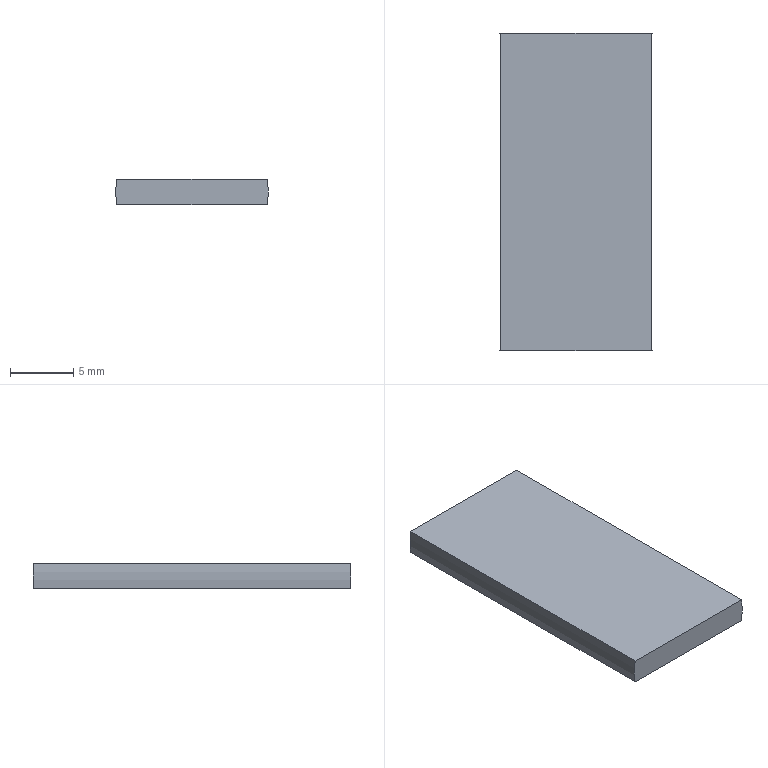Part | STEP file | Cooling fin - 2 - Tower - 1 cav | 1 solid | 6 faces | box 12 x 25 x 2 mm | volume 597.211 mm3 | plane 4 | cylinder 2 | commonest cylinder face diameters 12 x2
STEP:
#1=CARTESIAN_POINT('',(0.,0.,0.));
#2=DIRECTION('',(0.,0.,1.));
#3=DIRECTION('',(1.,0.,0.));
#4=AXIS2_PLACEMENT_3D('',#1,#2,#3);
#5=CARTESIAN_POINT('',(5.916,0.,-1.));
#6=VERTEX_POINT('',#5);
#7=CARTESIAN_POINT('',(5.916,25.,-1.));
#8=VERTEX_POINT('',#7);
#9=CARTESIAN_POINT('',(5.916,-15.,-1.));
#10=DIRECTION('',(0.,1.,0.));
#11=VECTOR('',#10,1.);
#12=LINE('',#9,#11);
#13=CARTESIAN_POINT('',(-7.5,25.,-1.));
#14=DIRECTION('',(0.,0.,1.));
#15=DIRECTION('',(1.,0.,0.));
#16=AXIS2_PLACEMENT_3D('',#13,#14,#15);
#17=PLANE('',#16);
#18=CARTESIAN_POINT('',(13.416,-40.));
#19=DIRECTION('',(0.,1.));
#20=VECTOR('',#19,1.);
#21=LINE('',#18,#20);
#22=(GEOMETRIC_REPRESENTATION_CONTEXT(2)PARAMETRIC_REPRESENTATION_CONTEXT()REPRESENTATION_CONTEXT('',''));
#23=DEFINITIONAL_REPRESENTATION('',(#21),#22);
#24=PCURVE('',#17,#23);
#25=CARTESIAN_POINT('',(0.,-15.,0.));
#26=DIRECTION('',(0.,1.,0.));
#27=DIRECTION('',(0.,0.,1.));
#28=AXIS2_PLACEMENT_3D('',#25,#26,#27);
#29=CYLINDRICAL_SURFACE('',#28,6.);
#30=CARTESIAN_POINT('',(1.738,0.));
#31=DIRECTION('',(0.,1.));
#32=VECTOR('',#31,1.);
#33=LINE('',#30,#32);
#34=(GEOMETRIC_REPRESENTATION_CONTEXT(2)PARAMETRIC_REPRESENTATION_CONTEXT()REPRESENTATION_CONTEXT('',''));
#35=DEFINITIONAL_REPRESENTATION('',(#33),#34);
#36=PCURVE('',#29,#35);
#37=SURFACE_CURVE('',#12,(#24,#36),.PCURVE_S1.);
#38=EDGE_CURVE('',#6,#8,#37,.T.);
#39=ORIENTED_EDGE('',*,*,#38,.F.);
#40=CARTESIAN_POINT('',(-5.916,0.,-1.));
#41=VERTEX_POINT('',#40);
#42=CARTESIAN_POINT('',(-7.5,0.,-1.));
#43=DIRECTION('',(-1.,0.,0.));
#44=VECTOR('',#43,1.);
#45=LINE('',#42,#44);
#46=CARTESIAN_POINT('',(0.,-25.));
#47=DIRECTION('',(-1.,0.));
#48=VECTOR('',#47,1.);
#49=LINE('',#46,#48);
#50=(GEOMETRIC_REPRESENTATION_CONTEXT(2)PARAMETRIC_REPRESENTATION_CONTEXT()REPRESENTATION_CONTEXT('',''));
#51=DEFINITIONAL_REPRESENTATION('',(#49),#50);
#52=PCURVE('',#17,#51);
#53=CARTESIAN_POINT('',(0.,0.,0.));
#54=DIRECTION('',(0.,-1.,0.));
#55=DIRECTION('',(0.,0.,-1.));
#56=AXIS2_PLACEMENT_3D('',#53,#54,#55);
#57=PLANE('',#56);
#58=CARTESIAN_POINT('',(1.,-7.5));
#59=DIRECTION('',(0.,-1.));
#60=VECTOR('',#59,1.);
#61=LINE('',#58,#60);
#62=(GEOMETRIC_REPRESENTATION_CONTEXT(2)PARAMETRIC_REPRESENTATION_CONTEXT()REPRESENTATION_CONTEXT('',''));
#63=DEFINITIONAL_REPRESENTATION('',(#61),#62);
#64=PCURVE('',#57,#63);
#65=SURFACE_CURVE('',#45,(#52,#64),.PCURVE_S1.);
#66=EDGE_CURVE('',#6,#41,#65,.T.);
#67=ORIENTED_EDGE('',*,*,#66,.T.);
#68=CARTESIAN_POINT('',(-5.916,25.,-1.));
#69=VERTEX_POINT('',#68);
#70=CARTESIAN_POINT('',(-5.916,-15.,-1.));
#71=DIRECTION('',(0.,-1.,0.));
#72=VECTOR('',#71,1.);
#73=LINE('',#70,#72);
#74=CARTESIAN_POINT('',(1.584,-40.));
#75=DIRECTION('',(0.,-1.));
#76=VECTOR('',#75,1.);
#77=LINE('',#74,#76);
#78=(GEOMETRIC_REPRESENTATION_CONTEXT(2)PARAMETRIC_REPRESENTATION_CONTEXT()REPRESENTATION_CONTEXT('',''));
#79=DEFINITIONAL_REPRESENTATION('',(#77),#78);
#80=PCURVE('',#17,#79);
#81=CARTESIAN_POINT('',(0.,-15.,0.));
#82=DIRECTION('',(0.,1.,0.));
#83=DIRECTION('',(0.,0.,1.));
#84=AXIS2_PLACEMENT_3D('',#81,#82,#83);
#85=CYLINDRICAL_SURFACE('',#84,6.);
#86=CARTESIAN_POINT('',(4.545,0.));
#87=DIRECTION('',(0.,-1.));
#88=VECTOR('',#87,1.);
#89=LINE('',#86,#88);
#90=(GEOMETRIC_REPRESENTATION_CONTEXT(2)PARAMETRIC_REPRESENTATION_CONTEXT()REPRESENTATION_CONTEXT('',''));
#91=DEFINITIONAL_REPRESENTATION('',(#89),#90);
#92=PCURVE('',#85,#91);
#93=SURFACE_CURVE('',#73,(#80,#92),.PCURVE_S1.);
#94=EDGE_CURVE('',#69,#41,#93,.T.);
#95=ORIENTED_EDGE('',*,*,#94,.F.);
#96=CARTESIAN_POINT('',(-7.5,25.,-1.));
#97=DIRECTION('',(-1.,0.,0.));
#98=VECTOR('',#97,1.);
#99=LINE('',#96,#98);
#100=CARTESIAN_POINT('',(0.,0.));
#101=DIRECTION('',(-1.,0.));
#102=VECTOR('',#101,1.);
#103=LINE('',#100,#102);
#104=(GEOMETRIC_REPRESENTATION_CONTEXT(2)PARAMETRIC_REPRESENTATION_CONTEXT()REPRESENTATION_CONTEXT('',''));
#105=DEFINITIONAL_REPRESENTATION('',(#103),#104);
#106=PCURVE('',#17,#105);
#107=CARTESIAN_POINT('',(0.,25.,0.));
#108=DIRECTION('',(0.,-1.,0.));
#109=DIRECTION('',(0.,0.,-1.));
#110=AXIS2_PLACEMENT_3D('',#107,#108,#109);
#111=PLANE('',#110);
#112=CARTESIAN_POINT('',(1.,-7.5));
#113=DIRECTION('',(0.,-1.));
#114=VECTOR('',#113,1.);
#115=LINE('',#112,#114);
#116=(GEOMETRIC_REPRESENTATION_CONTEXT(2)PARAMETRIC_REPRESENTATION_CONTEXT()REPRESENTATION_CONTEXT('',''));
#117=DEFINITIONAL_REPRESENTATION('',(#115),#116);
#118=PCURVE('',#111,#117);
#119=SURFACE_CURVE('',#99,(#106,#118),.PCURVE_S1.);
#120=EDGE_CURVE('',#8,#69,#119,.T.);
#121=ORIENTED_EDGE('',*,*,#120,.F.);
#122=EDGE_LOOP('',(#39,#67,#95,#121));
#123=FACE_BOUND('',#122,.T.);
#124=ADVANCED_FACE('',(#123),#17,.F.);
#125=CARTESIAN_POINT('',(-5.916,0.,1.));
#126=VERTEX_POINT('',#125);
#127=CARTESIAN_POINT('',(-5.916,25.,1.));
#128=VERTEX_POINT('',#127);
#129=CARTESIAN_POINT('',(-5.916,-15.,1.));
#130=DIRECTION('',(0.,1.,0.));
#131=VECTOR('',#130,1.);
#132=LINE('',#129,#131);
#133=CARTESIAN_POINT('',(-7.5,25.,1.));
#134=DIRECTION('',(0.,0.,-1.));
#135=DIRECTION('',(-1.,0.,0.));
#136=AXIS2_PLACEMENT_3D('',#133,#134,#135);
#137=PLANE('',#136);
#138=CARTESIAN_POINT('',(-1.584,-40.));
#139=DIRECTION('',(0.,1.));
#140=VECTOR('',#139,1.);
#141=LINE('',#138,#140);
#142=(GEOMETRIC_REPRESENTATION_CONTEXT(2)PARAMETRIC_REPRESENTATION_CONTEXT()REPRESENTATION_CONTEXT('',''));
#143=DEFINITIONAL_REPRESENTATION('',(#141),#142);
#144=PCURVE('',#137,#143);
#145=CARTESIAN_POINT('',(4.88,0.));
#146=DIRECTION('',(0.,1.));
#147=VECTOR('',#146,1.);
#148=LINE('',#145,#147);
#149=(GEOMETRIC_REPRESENTATION_CONTEXT(2)PARAMETRIC_REPRESENTATION_CONTEXT()REPRESENTATION_CONTEXT('',''));
#150=DEFINITIONAL_REPRESENTATION('',(#148),#149);
#151=PCURVE('',#85,#150);
#152=SURFACE_CURVE('',#132,(#144,#151),.PCURVE_S1.);
#153=EDGE_CURVE('',#126,#128,#152,.T.);
#154=ORIENTED_EDGE('',*,*,#153,.F.);
#155=CARTESIAN_POINT('',(5.916,0.,1.));
#156=VERTEX_POINT('',#155);
#157=CARTESIAN_POINT('',(-7.5,0.,1.));
#158=DIRECTION('',(1.,0.,0.));
#159=VECTOR('',#158,1.);
#160=LINE('',#157,#159);
#161=CARTESIAN_POINT('',(0.,-25.));
#162=DIRECTION('',(-1.,0.));
#163=VECTOR('',#162,1.);
#164=LINE('',#161,#163);
#165=(GEOMETRIC_REPRESENTATION_CONTEXT(2)PARAMETRIC_REPRESENTATION_CONTEXT()REPRESENTATION_CONTEXT('',''));
#166=DEFINITIONAL_REPRESENTATION('',(#164),#165);
#167=PCURVE('',#137,#166);
#168=CARTESIAN_POINT('',(-1.,-7.5));
#169=DIRECTION('',(0.,1.));
#170=VECTOR('',#169,1.);
#171=LINE('',#168,#170);
#172=(GEOMETRIC_REPRESENTATION_CONTEXT(2)PARAMETRIC_REPRESENTATION_CONTEXT()REPRESENTATION_CONTEXT('',''));
#173=DEFINITIONAL_REPRESENTATION('',(#171),#172);
#174=PCURVE('',#57,#173);
#175=SURFACE_CURVE('',#160,(#167,#174),.PCURVE_S1.);
#176=EDGE_CURVE('',#126,#156,#175,.T.);
#177=ORIENTED_EDGE('',*,*,#176,.T.);
#178=CARTESIAN_POINT('',(5.916,25.,1.));
#179=VERTEX_POINT('',#178);
#180=CARTESIAN_POINT('',(5.916,-15.,1.));
#181=DIRECTION('',(0.,-1.,0.));
#182=VECTOR('',#181,1.);
#183=LINE('',#180,#182);
#184=CARTESIAN_POINT('',(-13.416,-40.));
#185=DIRECTION('',(0.,-1.));
#186=VECTOR('',#185,1.);
#187=LINE('',#184,#186);
#188=(GEOMETRIC_REPRESENTATION_CONTEXT(2)PARAMETRIC_REPRESENTATION_CONTEXT()REPRESENTATION_CONTEXT('',''));
#189=DEFINITIONAL_REPRESENTATION('',(#187),#188);
#190=PCURVE('',#137,#189);
#191=CARTESIAN_POINT('',(1.403,0.));
#192=DIRECTION('',(0.,-1.));
#193=VECTOR('',#192,1.);
#194=LINE('',#191,#193);
#195=(GEOMETRIC_REPRESENTATION_CONTEXT(2)PARAMETRIC_REPRESENTATION_CONTEXT()REPRESENTATION_CONTEXT('',''));
#196=DEFINITIONAL_REPRESENTATION('',(#194),#195);
#197=PCURVE('',#29,#196);
#198=SURFACE_CURVE('',#183,(#190,#197),.PCURVE_S1.);
#199=EDGE_CURVE('',#179,#156,#198,.T.);
#200=ORIENTED_EDGE('',*,*,#199,.F.);
#201=CARTESIAN_POINT('',(-7.5,25.,1.));
#202=DIRECTION('',(1.,0.,0.));
#203=VECTOR('',#202,1.);
#204=LINE('',#201,#203);
#205=CARTESIAN_POINT('',(0.,0.));
#206=DIRECTION('',(-1.,0.));
#207=VECTOR('',#206,1.);
#208=LINE('',#205,#207);
#209=(GEOMETRIC_REPRESENTATION_CONTEXT(2)PARAMETRIC_REPRESENTATION_CONTEXT()REPRESENTATION_CONTEXT('',''));
#210=DEFINITIONAL_REPRESENTATION('',(#208),#209);
#211=PCURVE('',#137,#210);
#212=CARTESIAN_POINT('',(-1.,-7.5));
#213=DIRECTION('',(0.,1.));
#214=VECTOR('',#213,1.);
#215=LINE('',#212,#214);
#216=(GEOMETRIC_REPRESENTATION_CONTEXT(2)PARAMETRIC_REPRESENTATION_CONTEXT()REPRESENTATION_CONTEXT('',''));
#217=DEFINITIONAL_REPRESENTATION('',(#215),#216);
#218=PCURVE('',#111,#217);
#219=SURFACE_CURVE('',#204,(#211,#218),.PCURVE_S1.);
#220=EDGE_CURVE('',#128,#179,#219,.T.);
#221=ORIENTED_EDGE('',*,*,#220,.F.);
#222=EDGE_LOOP('',(#154,#177,#200,#221));
#223=FACE_BOUND('',#222,.T.);
#224=ADVANCED_FACE('',(#223),#137,.F.);
#225=CARTESIAN_POINT('',(0.,25.,0.));
#226=DIRECTION('',(0.,1.,0.));
#227=DIRECTION('',(0.,0.,1.));
#228=AXIS2_PLACEMENT_3D('',#225,#226,#227);
#229=CIRCLE('',#228,6.);
#230=CARTESIAN_POINT('',(-6.,0.));
#231=CARTESIAN_POINT('',(-6.,10.392));
#232=CARTESIAN_POINT('',(3.,5.196));
#233=CARTESIAN_POINT('',(12.,0.));
#234=CARTESIAN_POINT('',(3.,-5.196));
#235=CARTESIAN_POINT('',(-6.,-10.392));
#236=CARTESIAN_POINT('',(-6.,0.));
#237=(BOUNDED_CURVE()B_SPLINE_CURVE(2,(#230,#231,#232,#233,#234,#235,#236),.UNSPECIFIED.,.T.,.F.)B_SPLINE_CURVE_WITH_KNOTS((1,2,2,2,2,1),(-2.094,0.,2.094,4.189,6.283,8.378),.UNSPECIFIED.)CURVE()GEOMETRIC_REPRESENTATION_ITEM()RATIONAL_B_SPLINE_CURVE((1.,0.5,1.,0.5,1.,0.5,1.))REPRESENTATION_ITEM(''));
#238=(GEOMETRIC_REPRESENTATION_CONTEXT(2)PARAMETRIC_REPRESENTATION_CONTEXT()REPRESENTATION_CONTEXT('',''));
#239=DEFINITIONAL_REPRESENTATION('',(#237),#238);
#240=PCURVE('',#111,#239);
#241=CARTESIAN_POINT('',(0.,40.));
#242=DIRECTION('',(1.,0.));
#243=VECTOR('',#242,1.);
#244=LINE('',#241,#243);
#245=(GEOMETRIC_REPRESENTATION_CONTEXT(2)PARAMETRIC_REPRESENTATION_CONTEXT()REPRESENTATION_CONTEXT('',''));
#246=DEFINITIONAL_REPRESENTATION('',(#244),#245);
#247=PCURVE('',#29,#246);
#248=SURFACE_CURVE('',#229,(#240,#247),.PCURVE_S1.);
#249=EDGE_CURVE('',#179,#8,#248,.T.);
#250=ORIENTED_EDGE('',*,*,#249,.T.);
#251=ORIENTED_EDGE('',*,*,#120,.T.);
#252=CARTESIAN_POINT('',(0.,25.,0.));
#253=DIRECTION('',(0.,1.,0.));
#254=DIRECTION('',(0.,0.,1.));
#255=AXIS2_PLACEMENT_3D('',#252,#253,#254);
#256=CIRCLE('',#255,6.);
#257=CARTESIAN_POINT('',(-6.,0.));
#258=CARTESIAN_POINT('',(-6.,10.392));
#259=CARTESIAN_POINT('',(3.,5.196));
#260=CARTESIAN_POINT('',(12.,0.));
#261=CARTESIAN_POINT('',(3.,-5.196));
#262=CARTESIAN_POINT('',(-6.,-10.392));
#263=CARTESIAN_POINT('',(-6.,0.));
#264=(BOUNDED_CURVE()B_SPLINE_CURVE(2,(#257,#258,#259,#260,#261,#262,#263),.UNSPECIFIED.,.T.,.F.)B_SPLINE_CURVE_WITH_KNOTS((1,2,2,2,2,1),(-2.094,0.,2.094,4.189,6.283,8.378),.UNSPECIFIED.)CURVE()GEOMETRIC_REPRESENTATION_ITEM()RATIONAL_B_SPLINE_CURVE((1.,0.5,1.,0.5,1.,0.5,1.))REPRESENTATION_ITEM(''));
#265=(GEOMETRIC_REPRESENTATION_CONTEXT(2)PARAMETRIC_REPRESENTATION_CONTEXT()REPRESENTATION_CONTEXT('',''));
#266=DEFINITIONAL_REPRESENTATION('',(#264),#265);
#267=PCURVE('',#111,#266);
#268=CARTESIAN_POINT('',(0.,40.));
#269=DIRECTION('',(1.,0.));
#270=VECTOR('',#269,1.);
#271=LINE('',#268,#270);
#272=(GEOMETRIC_REPRESENTATION_CONTEXT(2)PARAMETRIC_REPRESENTATION_CONTEXT()REPRESENTATION_CONTEXT('',''));
#273=DEFINITIONAL_REPRESENTATION('',(#271),#272);
#274=PCURVE('',#85,#273);
#275=SURFACE_CURVE('',#256,(#267,#274),.PCURVE_S1.);
#276=EDGE_CURVE('',#69,#128,#275,.T.);
#277=ORIENTED_EDGE('',*,*,#276,.T.);
#278=ORIENTED_EDGE('',*,*,#220,.T.);
#279=EDGE_LOOP('',(#250,#251,#277,#278));
#280=FACE_BOUND('',#279,.T.);
#281=ADVANCED_FACE('',(#280),#111,.F.);
#282=ORIENTED_EDGE('',*,*,#66,.F.);
#283=CARTESIAN_POINT('',(0.,0.,0.));
#284=DIRECTION('',(0.,-1.,0.));
#285=DIRECTION('',(0.,0.,-1.));
#286=AXIS2_PLACEMENT_3D('',#283,#284,#285);
#287=CIRCLE('',#286,6.);
#288=CARTESIAN_POINT('',(0.,0.));
#289=DIRECTION('',(1.,0.));
#290=AXIS2_PLACEMENT_2D('',#288,#289);
#291=CIRCLE('',#290,6.);
#292=(GEOMETRIC_REPRESENTATION_CONTEXT(2)PARAMETRIC_REPRESENTATION_CONTEXT()REPRESENTATION_CONTEXT('',''));
#293=DEFINITIONAL_REPRESENTATION('',(#291),#292);
#294=PCURVE('',#57,#293);
#295=CARTESIAN_POINT('',(3.142,15.));
#296=DIRECTION('',(-1.,0.));
#297=VECTOR('',#296,1.);
#298=LINE('',#295,#297);
#299=(GEOMETRIC_REPRESENTATION_CONTEXT(2)PARAMETRIC_REPRESENTATION_CONTEXT()REPRESENTATION_CONTEXT('',''));
#300=DEFINITIONAL_REPRESENTATION('',(#298),#299);
#301=PCURVE('',#29,#300);
#302=SURFACE_CURVE('',#287,(#294,#301),.PCURVE_S1.);
#303=EDGE_CURVE('',#6,#156,#302,.T.);
#304=ORIENTED_EDGE('',*,*,#303,.T.);
#305=ORIENTED_EDGE('',*,*,#176,.F.);
#306=CARTESIAN_POINT('',(0.,0.,0.));
#307=DIRECTION('',(0.,-1.,0.));
#308=DIRECTION('',(0.,0.,-1.));
#309=AXIS2_PLACEMENT_3D('',#306,#307,#308);
#310=CIRCLE('',#309,6.);
#311=CARTESIAN_POINT('',(0.,0.));
#312=DIRECTION('',(1.,0.));
#313=AXIS2_PLACEMENT_2D('',#311,#312);
#314=CIRCLE('',#313,6.);
#315=(GEOMETRIC_REPRESENTATION_CONTEXT(2)PARAMETRIC_REPRESENTATION_CONTEXT()REPRESENTATION_CONTEXT('',''));
#316=DEFINITIONAL_REPRESENTATION('',(#314),#315);
#317=PCURVE('',#57,#316);
#318=CARTESIAN_POINT('',(9.425,15.));
#319=DIRECTION('',(-1.,0.));
#320=VECTOR('',#319,1.);
#321=LINE('',#318,#320);
#322=(GEOMETRIC_REPRESENTATION_CONTEXT(2)PARAMETRIC_REPRESENTATION_CONTEXT()REPRESENTATION_CONTEXT('',''));
#323=DEFINITIONAL_REPRESENTATION('',(#321),#322);
#324=PCURVE('',#85,#323);
#325=SURFACE_CURVE('',#310,(#317,#324),.PCURVE_S1.);
#326=EDGE_CURVE('',#126,#41,#325,.T.);
#327=ORIENTED_EDGE('',*,*,#326,.T.);
#328=EDGE_LOOP('',(#282,#304,#305,#327));
#329=FACE_BOUND('',#328,.T.);
#330=ADVANCED_FACE('',(#329),#57,.T.);
#331=ORIENTED_EDGE('',*,*,#94,.T.);
#332=ORIENTED_EDGE('',*,*,#326,.F.);
#333=ORIENTED_EDGE('',*,*,#153,.T.);
#334=ORIENTED_EDGE('',*,*,#276,.F.);
#335=EDGE_LOOP('',(#331,#332,#333,#334));
#336=FACE_BOUND('',#335,.T.);
#337=ADVANCED_FACE('',(#336),#85,.T.);
#338=ORIENTED_EDGE('',*,*,#38,.T.);
#339=ORIENTED_EDGE('',*,*,#249,.F.);
#340=ORIENTED_EDGE('',*,*,#199,.T.);
#341=ORIENTED_EDGE('',*,*,#303,.F.);
#342=EDGE_LOOP('',(#338,#339,#340,#341));
#343=FACE_BOUND('',#342,.T.);
#344=ADVANCED_FACE('',(#343),#29,.T.);
#345=CLOSED_SHELL('',(#124,#224,#281,#330,#337,#344));
#346=MANIFOLD_SOLID_BREP('',#345);
#347=(LENGTH_UNIT()NAMED_UNIT(*)SI_UNIT(.MILLI.,.METRE.));
#348=UNCERTAINTY_MEASURE_WITH_UNIT(LENGTH_MEASURE(0.0000001),#347,'','');
#349=(NAMED_UNIT(*)PLANE_ANGLE_UNIT()SI_UNIT($,.RADIAN.));
#350=(NAMED_UNIT(*)SI_UNIT($,.STERADIAN.)SOLID_ANGLE_UNIT());
#351=(GEOMETRIC_REPRESENTATION_CONTEXT(3)GLOBAL_UNCERTAINTY_ASSIGNED_CONTEXT((#348))GLOBAL_UNIT_ASSIGNED_CONTEXT((#347,#349,#350))REPRESENTATION_CONTEXT('',''));
#352=ADVANCED_BREP_SHAPE_REPRESENTATION('',(#4,#346),#351);